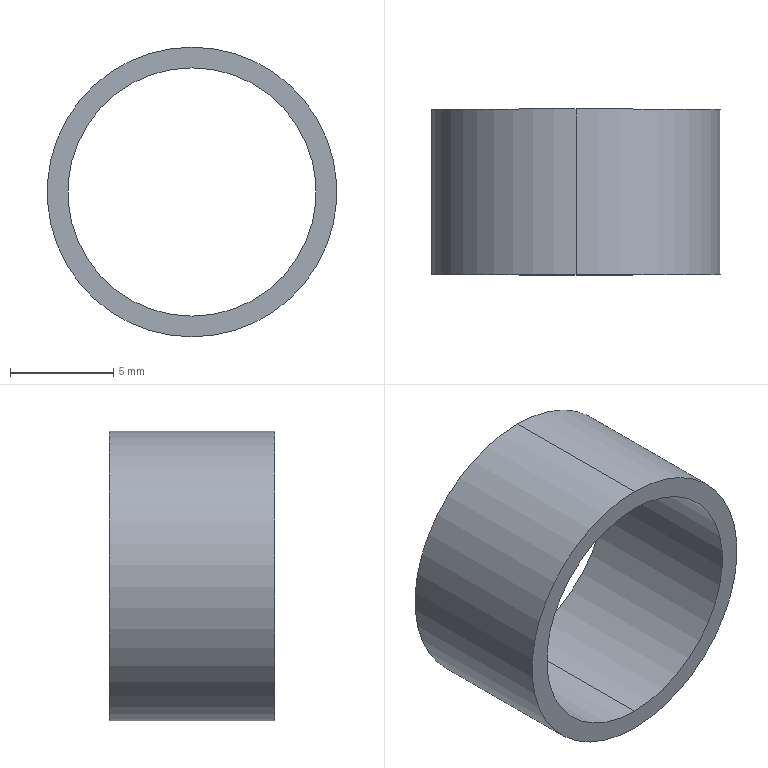Part | SolidWorks | features Extrusion 1 | 1 solid | 6 faces | box 14 x 8 x 14 mm | volume 326.726 mm3 | cylinder 4 | plane 2 | commonest cylinder face diameters 12 x2 14 x2
STEP:
#1=CARTESIAN_POINT('',(0.,8.,-6.));
#2=VERTEX_POINT('',#1);
#3=CARTESIAN_POINT('',(0.,8.,6.));
#4=VERTEX_POINT('',#3);
#5=CARTESIAN_POINT('',(0.,8.,0.));
#6=DIRECTION('',(0.,1.,0.));
#7=DIRECTION('',(0.,0.,1.));
#8=AXIS2_PLACEMENT_3D('',#5,#6,#7);
#9=CIRCLE('',#8,6.);
#10=EDGE_CURVE('',#2,#4,#9,.T.);
#11=ORIENTED_EDGE('',*,*,#10,.T.);
#12=CARTESIAN_POINT('',(0.,0.,6.));
#13=VERTEX_POINT('',#12);
#14=CARTESIAN_POINT('',(0.,8.,6.));
#15=DIRECTION('',(0.,-1.,0.));
#16=VECTOR('',#15,1000.);
#17=LINE('',#14,#16);
#18=EDGE_CURVE('',#4,#13,#17,.T.);
#19=ORIENTED_EDGE('',*,*,#18,.T.);
#20=CARTESIAN_POINT('',(0.,0.,-6.));
#21=VERTEX_POINT('',#20);
#22=CARTESIAN_POINT('',(0.,0.,0.));
#23=DIRECTION('',(0.,1.,0.));
#24=DIRECTION('',(0.,0.,1.));
#25=AXIS2_PLACEMENT_3D('',#22,#23,#24);
#26=CIRCLE('',#25,6.);
#27=EDGE_CURVE('',#21,#13,#26,.T.);
#28=ORIENTED_EDGE('',*,*,#27,.F.);
#29=CARTESIAN_POINT('',(0.,8.,-6.));
#30=DIRECTION('',(0.,-1.,0.));
#31=VECTOR('',#30,1000.);
#32=LINE('',#29,#31);
#33=EDGE_CURVE('',#2,#21,#32,.T.);
#34=ORIENTED_EDGE('',*,*,#33,.F.);
#35=EDGE_LOOP('',(#11,#19,#28,#34));
#36=FACE_OUTER_BOUND('',#35,.T.);
#37=CARTESIAN_POINT('',(0.,8.,0.));
#38=DIRECTION('',(0.,-1.,0.));
#39=DIRECTION('',(0.,0.,-1.));
#40=AXIS2_PLACEMENT_3D('',#37,#38,#39);
#41=CYLINDRICAL_SURFACE('',#40,6.);
#42=ADVANCED_FACE('',(#36),#41,.F.);
#43=CARTESIAN_POINT('',(0.,8.,7.));
#44=VERTEX_POINT('',#43);
#45=CARTESIAN_POINT('',(0.,8.,-7.));
#46=VERTEX_POINT('',#45);
#47=CARTESIAN_POINT('',(0.,8.,0.));
#48=DIRECTION('',(0.,1.,0.));
#49=DIRECTION('',(0.,0.,1.));
#50=AXIS2_PLACEMENT_3D('',#47,#48,#49);
#51=CIRCLE('',#50,7.);
#52=EDGE_CURVE('',#44,#46,#51,.T.);
#53=ORIENTED_EDGE('',*,*,#52,.F.);
#54=CARTESIAN_POINT('',(0.,0.,7.));
#55=VERTEX_POINT('',#54);
#56=CARTESIAN_POINT('',(0.,8.,7.));
#57=DIRECTION('',(0.,-1.,0.));
#58=VECTOR('',#57,1000.);
#59=LINE('',#56,#58);
#60=EDGE_CURVE('',#44,#55,#59,.T.);
#61=ORIENTED_EDGE('',*,*,#60,.T.);
#62=CARTESIAN_POINT('',(0.,0.,-7.));
#63=VERTEX_POINT('',#62);
#64=CARTESIAN_POINT('',(0.,0.,0.));
#65=DIRECTION('',(0.,1.,0.));
#66=DIRECTION('',(0.,0.,1.));
#67=AXIS2_PLACEMENT_3D('',#64,#65,#66);
#68=CIRCLE('',#67,7.);
#69=EDGE_CURVE('',#55,#63,#68,.T.);
#70=ORIENTED_EDGE('',*,*,#69,.T.);
#71=CARTESIAN_POINT('',(0.,8.,-7.));
#72=DIRECTION('',(0.,-1.,0.));
#73=VECTOR('',#72,1000.);
#74=LINE('',#71,#73);
#75=EDGE_CURVE('',#46,#63,#74,.T.);
#76=ORIENTED_EDGE('',*,*,#75,.F.);
#77=EDGE_LOOP('',(#53,#61,#70,#76));
#78=FACE_OUTER_BOUND('',#77,.T.);
#79=CARTESIAN_POINT('',(0.,8.,0.));
#80=DIRECTION('',(0.,-1.,0.));
#81=DIRECTION('',(0.,0.,-1.));
#82=AXIS2_PLACEMENT_3D('',#79,#80,#81);
#83=CYLINDRICAL_SURFACE('',#82,7.);
#84=ADVANCED_FACE('',(#78),#83,.T.);
#85=CARTESIAN_POINT('',(0.,8.,0.));
#86=DIRECTION('',(0.,1.,0.));
#87=DIRECTION('',(0.,0.,1.));
#88=AXIS2_PLACEMENT_3D('',#85,#86,#87);
#89=CIRCLE('',#88,7.);
#90=EDGE_CURVE('',#46,#44,#89,.T.);
#91=ORIENTED_EDGE('',*,*,#90,.T.);
#92=ORIENTED_EDGE('',*,*,#52,.T.);
#93=EDGE_LOOP('',(#91,#92));
#94=FACE_OUTER_BOUND('',#93,.T.);
#95=ORIENTED_EDGE('',*,*,#10,.F.);
#96=CARTESIAN_POINT('',(0.,8.,0.));
#97=DIRECTION('',(0.,1.,0.));
#98=DIRECTION('',(0.,0.,1.));
#99=AXIS2_PLACEMENT_3D('',#96,#97,#98);
#100=CIRCLE('',#99,6.);
#101=EDGE_CURVE('',#4,#2,#100,.T.);
#102=ORIENTED_EDGE('',*,*,#101,.F.);
#103=EDGE_LOOP('',(#95,#102));
#104=FACE_BOUND('',#103,.T.);
#105=CARTESIAN_POINT('',(0.,8.,0.));
#106=DIRECTION('',(0.,1.,0.));
#107=DIRECTION('',(0.,0.,1.));
#108=AXIS2_PLACEMENT_3D('',#105,#106,#107);
#109=PLANE('',#108);
#110=ADVANCED_FACE('',(#94,#104),#109,.T.);
#111=CARTESIAN_POINT('',(0.,0.,0.));
#112=DIRECTION('',(0.,1.,0.));
#113=DIRECTION('',(0.,0.,1.));
#114=AXIS2_PLACEMENT_3D('',#111,#112,#113);
#115=CIRCLE('',#114,7.);
#116=EDGE_CURVE('',#63,#55,#115,.T.);
#117=ORIENTED_EDGE('',*,*,#116,.F.);
#118=ORIENTED_EDGE('',*,*,#69,.F.);
#119=EDGE_LOOP('',(#117,#118));
#120=FACE_OUTER_BOUND('',#119,.T.);
#121=ORIENTED_EDGE('',*,*,#27,.T.);
#122=CARTESIAN_POINT('',(0.,0.,0.));
#123=DIRECTION('',(0.,1.,0.));
#124=DIRECTION('',(0.,0.,1.));
#125=AXIS2_PLACEMENT_3D('',#122,#123,#124);
#126=CIRCLE('',#125,6.);
#127=EDGE_CURVE('',#13,#21,#126,.T.);
#128=ORIENTED_EDGE('',*,*,#127,.T.);
#129=EDGE_LOOP('',(#121,#128));
#130=FACE_BOUND('',#129,.T.);
#131=CARTESIAN_POINT('',(0.,0.,0.));
#132=DIRECTION('',(0.,1.,0.));
#133=DIRECTION('',(0.,0.,1.));
#134=AXIS2_PLACEMENT_3D('',#131,#132,#133);
#135=PLANE('',#134);
#136=ADVANCED_FACE('',(#120,#130),#135,.F.);
#137=ORIENTED_EDGE('',*,*,#60,.F.);
#138=ORIENTED_EDGE('',*,*,#90,.F.);
#139=ORIENTED_EDGE('',*,*,#75,.T.);
#140=ORIENTED_EDGE('',*,*,#116,.T.);
#141=EDGE_LOOP('',(#137,#138,#139,#140));
#142=FACE_OUTER_BOUND('',#141,.T.);
#143=CARTESIAN_POINT('',(0.,8.,0.));
#144=DIRECTION('',(0.,-1.,0.));
#145=DIRECTION('',(0.,0.,-1.));
#146=AXIS2_PLACEMENT_3D('',#143,#144,#145);
#147=CYLINDRICAL_SURFACE('',#146,7.);
#148=ADVANCED_FACE('',(#142),#147,.T.);
#149=ORIENTED_EDGE('',*,*,#18,.F.);
#150=ORIENTED_EDGE('',*,*,#101,.T.);
#151=ORIENTED_EDGE('',*,*,#33,.T.);
#152=ORIENTED_EDGE('',*,*,#127,.F.);
#153=EDGE_LOOP('',(#149,#150,#151,#152));
#154=FACE_OUTER_BOUND('',#153,.T.);
#155=CARTESIAN_POINT('',(0.,8.,0.));
#156=DIRECTION('',(0.,-1.,0.));
#157=DIRECTION('',(0.,0.,-1.));
#158=AXIS2_PLACEMENT_3D('',#155,#156,#157);
#159=CYLINDRICAL_SURFACE('',#158,6.);
#160=ADVANCED_FACE('',(#154),#159,.F.);
#161=CLOSED_SHELL('',(#42,#84,#110,#136,#148,#160));
#162=MANIFOLD_SOLID_BREP('',#161);
#163=CARTESIAN_POINT('',(0.,0.,0.));
#164=DIRECTION('',(0.,0.,1.));
#165=DIRECTION('',(1.,0.,0.));
#166=AXIS2_PLACEMENT_3D('',#163,#164,#165);
#167=(LENGTH_UNIT()NAMED_UNIT(*)SI_UNIT(.MILLI.,.METRE.));
#168=UNCERTAINTY_MEASURE_WITH_UNIT(LENGTH_MEASURE(0.00001),#167,'','');
#169=(NAMED_UNIT(*)PLANE_ANGLE_UNIT()SI_UNIT($,.RADIAN.));
#170=(NAMED_UNIT(*)SI_UNIT($,.STERADIAN.)SOLID_ANGLE_UNIT());
#171=(GEOMETRIC_REPRESENTATION_CONTEXT(3)GLOBAL_UNCERTAINTY_ASSIGNED_CONTEXT((#168))GLOBAL_UNIT_ASSIGNED_CONTEXT((#167,#169,#170))REPRESENTATION_CONTEXT('',''));
#172=ADVANCED_BREP_SHAPE_REPRESENTATION('',(#162,#166),#171);